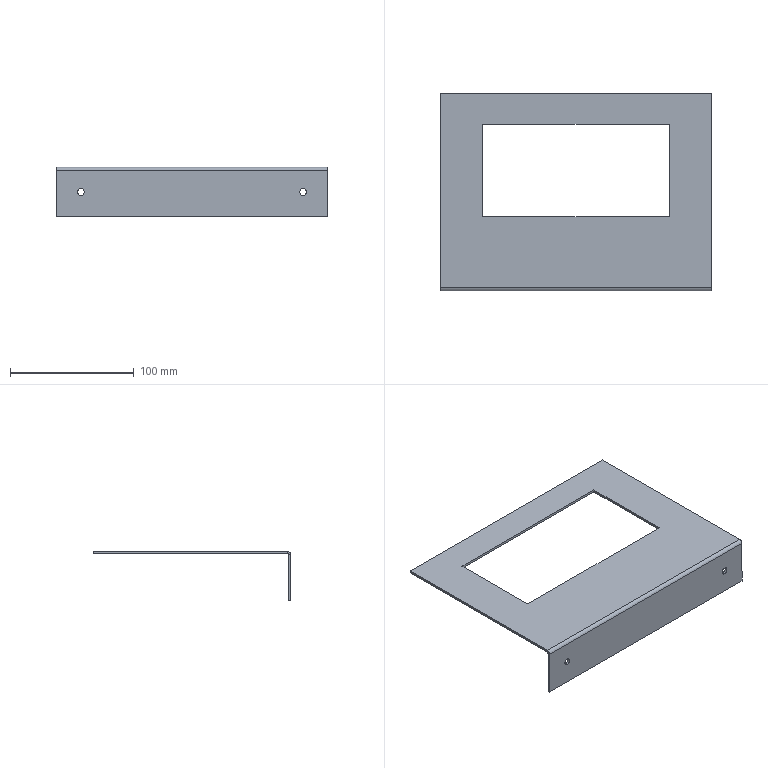Part | STEP file | 1 solid | 22 faces | box 220 x 160 x 40 mm | volume 64047 mm3 | plane 16 | cylinder 6 | commonest cylinder face diameters 5.5 x4 1.473 x1 5.473 x1
STEP:
#1=CARTESIAN_POINT('',(0.,0.,0.));
#2=DIRECTION('',(0.,0.,1.));
#3=DIRECTION('',(1.,0.,0.));
#4=AXIS2_PLACEMENT_3D('',#1,#2,#3);
#5=CARTESIAN_POINT('',(200.,0.,-17.25));
#6=VERTEX_POINT('',#5);
#7=CARTESIAN_POINT('',(200.,2.,-17.25));
#8=VERTEX_POINT('',#7);
#9=CARTESIAN_POINT('',(200.,2.,-17.25));
#10=DIRECTION('',(0.,1.,0.));
#11=VECTOR('',#10,1.);
#12=LINE('',#9,#11);
#13=CARTESIAN_POINT('',(200.,2.,-20.));
#14=DIRECTION('',(0.,1.,0.));
#15=DIRECTION('',(0.,0.,1.));
#16=AXIS2_PLACEMENT_3D('',#13,#14,#15);
#17=CYLINDRICAL_SURFACE('',#16,2.75);
#18=CARTESIAN_POINT('',(6.283,0.));
#19=DIRECTION('',(0.,1.));
#20=VECTOR('',#19,1.);
#21=LINE('',#18,#20);
#22=(GEOMETRIC_REPRESENTATION_CONTEXT(2)PARAMETRIC_REPRESENTATION_CONTEXT()REPRESENTATION_CONTEXT('',''));
#23=DEFINITIONAL_REPRESENTATION('',(#21),#22);
#24=PCURVE('',#17,#23);
#25=CARTESIAN_POINT('',(200.,2.,-20.));
#26=DIRECTION('',(0.,1.,0.));
#27=DIRECTION('',(0.,0.,1.));
#28=AXIS2_PLACEMENT_3D('',#25,#26,#27);
#29=CYLINDRICAL_SURFACE('',#28,2.75);
#30=CARTESIAN_POINT('',(0.,0.));
#31=DIRECTION('',(0.,1.));
#32=VECTOR('',#31,1.);
#33=LINE('',#30,#32);
#34=(GEOMETRIC_REPRESENTATION_CONTEXT(2)PARAMETRIC_REPRESENTATION_CONTEXT()REPRESENTATION_CONTEXT('',''));
#35=DEFINITIONAL_REPRESENTATION('',(#33),#34);
#36=PCURVE('',#29,#35);
#37=SURFACE_CURVE('',#12,(#24,#36),.PCURVE_S1.);
#38=EDGE_CURVE('',#6,#8,#37,.T.);
#39=ORIENTED_EDGE('',*,*,#38,.T.);
#40=CARTESIAN_POINT('',(200.,2.,-22.75));
#41=VERTEX_POINT('',#40);
#42=CARTESIAN_POINT('',(200.,2.,-20.));
#43=DIRECTION('',(0.,1.,0.));
#44=DIRECTION('',(0.,0.,1.));
#45=AXIS2_PLACEMENT_3D('',#42,#43,#44);
#46=CIRCLE('',#45,2.75);
#47=CARTESIAN_POINT('',(0.,0.));
#48=DIRECTION('',(1.,0.));
#49=VECTOR('',#48,1.);
#50=LINE('',#47,#49);
#51=(GEOMETRIC_REPRESENTATION_CONTEXT(2)PARAMETRIC_REPRESENTATION_CONTEXT()REPRESENTATION_CONTEXT('',''));
#52=DEFINITIONAL_REPRESENTATION('',(#50),#51);
#53=PCURVE('',#17,#52);
#54=CARTESIAN_POINT('',(0.,2.,0.));
#55=DIRECTION('',(0.,1.,0.));
#56=DIRECTION('',(0.,0.,1.));
#57=AXIS2_PLACEMENT_3D('',#54,#55,#56);
#58=PLANE('',#57);
#59=CARTESIAN_POINT('',(-20.,200.));
#60=DIRECTION('',(1.,0.));
#61=AXIS2_PLACEMENT_2D('',#59,#60);
#62=CIRCLE('',#61,2.75);
#63=(GEOMETRIC_REPRESENTATION_CONTEXT(2)PARAMETRIC_REPRESENTATION_CONTEXT()REPRESENTATION_CONTEXT('',''));
#64=DEFINITIONAL_REPRESENTATION('',(#62),#63);
#65=PCURVE('',#58,#64);
#66=SURFACE_CURVE('',#46,(#53,#65),.PCURVE_S1.);
#67=EDGE_CURVE('',#41,#8,#66,.T.);
#68=ORIENTED_EDGE('',*,*,#67,.F.);
#69=CARTESIAN_POINT('',(200.,0.,-22.75));
#70=VERTEX_POINT('',#69);
#71=CARTESIAN_POINT('',(200.,2.,-22.75));
#72=DIRECTION('',(0.,1.,0.));
#73=VECTOR('',#72,1.);
#74=LINE('',#71,#73);
#75=CARTESIAN_POINT('',(3.142,0.));
#76=DIRECTION('',(0.,1.));
#77=VECTOR('',#76,1.);
#78=LINE('',#75,#77);
#79=(GEOMETRIC_REPRESENTATION_CONTEXT(2)PARAMETRIC_REPRESENTATION_CONTEXT()REPRESENTATION_CONTEXT('',''));
#80=DEFINITIONAL_REPRESENTATION('',(#78),#79);
#81=PCURVE('',#17,#80);
#82=CARTESIAN_POINT('',(3.142,0.));
#83=DIRECTION('',(0.,1.));
#84=VECTOR('',#83,1.);
#85=LINE('',#82,#84);
#86=(GEOMETRIC_REPRESENTATION_CONTEXT(2)PARAMETRIC_REPRESENTATION_CONTEXT()REPRESENTATION_CONTEXT('',''));
#87=DEFINITIONAL_REPRESENTATION('',(#85),#86);
#88=PCURVE('',#29,#87);
#89=SURFACE_CURVE('',#74,(#81,#88),.PCURVE_S1.);
#90=EDGE_CURVE('',#70,#41,#89,.T.);
#91=ORIENTED_EDGE('',*,*,#90,.F.);
#92=CARTESIAN_POINT('',(200.,0.,-20.));
#93=DIRECTION('',(0.,1.,0.));
#94=DIRECTION('',(0.,0.,1.));
#95=AXIS2_PLACEMENT_3D('',#92,#93,#94);
#96=CIRCLE('',#95,2.75);
#97=CARTESIAN_POINT('',(0.,-2.));
#98=DIRECTION('',(1.,0.));
#99=VECTOR('',#98,1.);
#100=LINE('',#97,#99);
#101=(GEOMETRIC_REPRESENTATION_CONTEXT(2)PARAMETRIC_REPRESENTATION_CONTEXT()REPRESENTATION_CONTEXT('',''));
#102=DEFINITIONAL_REPRESENTATION('',(#100),#101);
#103=PCURVE('',#17,#102);
#104=CARTESIAN_POINT('',(0.,0.,0.));
#105=DIRECTION('',(0.,1.,0.));
#106=DIRECTION('',(0.,0.,1.));
#107=AXIS2_PLACEMENT_3D('',#104,#105,#106);
#108=PLANE('',#107);
#109=CARTESIAN_POINT('',(-20.,200.));
#110=DIRECTION('',(1.,0.));
#111=AXIS2_PLACEMENT_2D('',#109,#110);
#112=CIRCLE('',#111,2.75);
#113=(GEOMETRIC_REPRESENTATION_CONTEXT(2)PARAMETRIC_REPRESENTATION_CONTEXT()REPRESENTATION_CONTEXT('',''));
#114=DEFINITIONAL_REPRESENTATION('',(#112),#113);
#115=PCURVE('',#108,#114);
#116=SURFACE_CURVE('',#96,(#103,#115),.PCURVE_S1.);
#117=EDGE_CURVE('',#70,#6,#116,.T.);
#118=ORIENTED_EDGE('',*,*,#117,.T.);
#119=EDGE_LOOP('',(#39,#68,#91,#118));
#120=FACE_BOUND('',#119,.F.);
#121=ADVANCED_FACE('',(#120),#17,.F.);
#122=CARTESIAN_POINT('',(20.,0.,-17.25));
#123=VERTEX_POINT('',#122);
#124=CARTESIAN_POINT('',(20.,2.,-17.25));
#125=VERTEX_POINT('',#124);
#126=CARTESIAN_POINT('',(20.,2.,-17.25));
#127=DIRECTION('',(0.,1.,0.));
#128=VECTOR('',#127,1.);
#129=LINE('',#126,#128);
#130=CARTESIAN_POINT('',(20.,2.,-20.));
#131=DIRECTION('',(0.,1.,0.));
#132=DIRECTION('',(0.,0.,1.));
#133=AXIS2_PLACEMENT_3D('',#130,#131,#132);
#134=CYLINDRICAL_SURFACE('',#133,2.75);
#135=CARTESIAN_POINT('',(6.283,0.));
#136=DIRECTION('',(0.,1.));
#137=VECTOR('',#136,1.);
#138=LINE('',#135,#137);
#139=(GEOMETRIC_REPRESENTATION_CONTEXT(2)PARAMETRIC_REPRESENTATION_CONTEXT()REPRESENTATION_CONTEXT('',''));
#140=DEFINITIONAL_REPRESENTATION('',(#138),#139);
#141=PCURVE('',#134,#140);
#142=CARTESIAN_POINT('',(20.,2.,-20.));
#143=DIRECTION('',(0.,1.,0.));
#144=DIRECTION('',(0.,0.,1.));
#145=AXIS2_PLACEMENT_3D('',#142,#143,#144);
#146=CYLINDRICAL_SURFACE('',#145,2.75);
#147=CARTESIAN_POINT('',(0.,0.));
#148=DIRECTION('',(0.,1.));
#149=VECTOR('',#148,1.);
#150=LINE('',#147,#149);
#151=(GEOMETRIC_REPRESENTATION_CONTEXT(2)PARAMETRIC_REPRESENTATION_CONTEXT()REPRESENTATION_CONTEXT('',''));
#152=DEFINITIONAL_REPRESENTATION('',(#150),#151);
#153=PCURVE('',#146,#152);
#154=SURFACE_CURVE('',#129,(#141,#153),.PCURVE_S1.);
#155=EDGE_CURVE('',#123,#125,#154,.T.);
#156=ORIENTED_EDGE('',*,*,#155,.T.);
#157=CARTESIAN_POINT('',(20.,2.,-22.75));
#158=VERTEX_POINT('',#157);
#159=CARTESIAN_POINT('',(20.,2.,-20.));
#160=DIRECTION('',(0.,1.,0.));
#161=DIRECTION('',(0.,0.,1.));
#162=AXIS2_PLACEMENT_3D('',#159,#160,#161);
#163=CIRCLE('',#162,2.75);
#164=CARTESIAN_POINT('',(0.,0.));
#165=DIRECTION('',(1.,0.));
#166=VECTOR('',#165,1.);
#167=LINE('',#164,#166);
#168=(GEOMETRIC_REPRESENTATION_CONTEXT(2)PARAMETRIC_REPRESENTATION_CONTEXT()REPRESENTATION_CONTEXT('',''));
#169=DEFINITIONAL_REPRESENTATION('',(#167),#168);
#170=PCURVE('',#134,#169);
#171=CARTESIAN_POINT('',(-20.,20.));
#172=DIRECTION('',(1.,0.));
#173=AXIS2_PLACEMENT_2D('',#171,#172);
#174=CIRCLE('',#173,2.75);
#175=(GEOMETRIC_REPRESENTATION_CONTEXT(2)PARAMETRIC_REPRESENTATION_CONTEXT()REPRESENTATION_CONTEXT('',''));
#176=DEFINITIONAL_REPRESENTATION('',(#174),#175);
#177=PCURVE('',#58,#176);
#178=SURFACE_CURVE('',#163,(#170,#177),.PCURVE_S1.);
#179=EDGE_CURVE('',#158,#125,#178,.T.);
#180=ORIENTED_EDGE('',*,*,#179,.F.);
#181=CARTESIAN_POINT('',(20.,0.,-22.75));
#182=VERTEX_POINT('',#181);
#183=CARTESIAN_POINT('',(20.,2.,-22.75));
#184=DIRECTION('',(0.,1.,0.));
#185=VECTOR('',#184,1.);
#186=LINE('',#183,#185);
#187=CARTESIAN_POINT('',(3.142,0.));
#188=DIRECTION('',(0.,1.));
#189=VECTOR('',#188,1.);
#190=LINE('',#187,#189);
#191=(GEOMETRIC_REPRESENTATION_CONTEXT(2)PARAMETRIC_REPRESENTATION_CONTEXT()REPRESENTATION_CONTEXT('',''));
#192=DEFINITIONAL_REPRESENTATION('',(#190),#191);
#193=PCURVE('',#134,#192);
#194=CARTESIAN_POINT('',(3.142,0.));
#195=DIRECTION('',(0.,1.));
#196=VECTOR('',#195,1.);
#197=LINE('',#194,#196);
#198=(GEOMETRIC_REPRESENTATION_CONTEXT(2)PARAMETRIC_REPRESENTATION_CONTEXT()REPRESENTATION_CONTEXT('',''));
#199=DEFINITIONAL_REPRESENTATION('',(#197),#198);
#200=PCURVE('',#146,#199);
#201=SURFACE_CURVE('',#186,(#193,#200),.PCURVE_S1.);
#202=EDGE_CURVE('',#182,#158,#201,.T.);
#203=ORIENTED_EDGE('',*,*,#202,.F.);
#204=CARTESIAN_POINT('',(20.,0.,-20.));
#205=DIRECTION('',(0.,1.,0.));
#206=DIRECTION('',(0.,0.,1.));
#207=AXIS2_PLACEMENT_3D('',#204,#205,#206);
#208=CIRCLE('',#207,2.75);
#209=CARTESIAN_POINT('',(0.,-2.));
#210=DIRECTION('',(1.,0.));
#211=VECTOR('',#210,1.);
#212=LINE('',#209,#211);
#213=(GEOMETRIC_REPRESENTATION_CONTEXT(2)PARAMETRIC_REPRESENTATION_CONTEXT()REPRESENTATION_CONTEXT('',''));
#214=DEFINITIONAL_REPRESENTATION('',(#212),#213);
#215=PCURVE('',#134,#214);
#216=CARTESIAN_POINT('',(-20.,20.));
#217=DIRECTION('',(1.,0.));
#218=AXIS2_PLACEMENT_2D('',#216,#217);
#219=CIRCLE('',#218,2.75);
#220=(GEOMETRIC_REPRESENTATION_CONTEXT(2)PARAMETRIC_REPRESENTATION_CONTEXT()REPRESENTATION_CONTEXT('',''));
#221=DEFINITIONAL_REPRESENTATION('',(#219),#220);
#222=PCURVE('',#108,#221);
#223=SURFACE_CURVE('',#208,(#215,#222),.PCURVE_S1.);
#224=EDGE_CURVE('',#182,#123,#223,.T.);
#225=ORIENTED_EDGE('',*,*,#224,.T.);
#226=EDGE_LOOP('',(#156,#180,#203,#225));
#227=FACE_BOUND('',#226,.F.);
#228=ADVANCED_FACE('',(#227),#134,.F.);
#229=CARTESIAN_POINT('',(0.,160.,-2.));
#230=VERTEX_POINT('',#229);
#231=CARTESIAN_POINT('',(0.,2.737,-2.));
#232=VERTEX_POINT('',#231);
#233=CARTESIAN_POINT('',(0.,0.,-2.));
#234=DIRECTION('',(0.,-1.,0.));
#235=VECTOR('',#234,1.);
#236=LINE('',#233,#235);
#237=CARTESIAN_POINT('',(0.,0.,-2.));
#238=DIRECTION('',(-1.,0.,0.));
#239=DIRECTION('',(0.,0.,1.));
#240=AXIS2_PLACEMENT_3D('',#237,#238,#239);
#241=PLANE('',#240);
#242=CARTESIAN_POINT('',(0.,0.));
#243=DIRECTION('',(0.,-1.));
#244=VECTOR('',#243,1.);
#245=LINE('',#242,#244);
#246=(GEOMETRIC_REPRESENTATION_CONTEXT(2)PARAMETRIC_REPRESENTATION_CONTEXT()REPRESENTATION_CONTEXT('',''));
#247=DEFINITIONAL_REPRESENTATION('',(#245),#246);
#248=PCURVE('',#241,#247);
#249=CARTESIAN_POINT('',(0.,0.,-2.));
#250=DIRECTION('',(0.,0.,-1.));
#251=DIRECTION('',(-1.,0.,0.));
#252=AXIS2_PLACEMENT_3D('',#249,#250,#251);
#253=PLANE('',#252);
#254=CARTESIAN_POINT('',(0.,0.));
#255=DIRECTION('',(0.,-1.));
#256=VECTOR('',#255,1.);
#257=LINE('',#254,#256);
#258=(GEOMETRIC_REPRESENTATION_CONTEXT(2)PARAMETRIC_REPRESENTATION_CONTEXT()REPRESENTATION_CONTEXT('',''));
#259=DEFINITIONAL_REPRESENTATION('',(#257),#258);
#260=PCURVE('',#253,#259);
#261=SURFACE_CURVE('',#236,(#248,#260),.PCURVE_S1.);
#262=EDGE_CURVE('',#230,#232,#261,.T.);
#263=ORIENTED_EDGE('',*,*,#262,.T.);
#264=CARTESIAN_POINT('',(0.,2.737,0.));
#265=VERTEX_POINT('',#264);
#266=CARTESIAN_POINT('',(0.,2.737,-2.));
#267=DIRECTION('',(0.,0.,1.));
#268=VECTOR('',#267,1.);
#269=LINE('',#266,#268);
#270=CARTESIAN_POINT('',(0.,2.737));
#271=DIRECTION('',(1.,0.));
#272=VECTOR('',#271,1.);
#273=LINE('',#270,#272);
#274=(GEOMETRIC_REPRESENTATION_CONTEXT(2)PARAMETRIC_REPRESENTATION_CONTEXT()REPRESENTATION_CONTEXT('',''));
#275=DEFINITIONAL_REPRESENTATION('',(#273),#274);
#276=PCURVE('',#241,#275);
#277=CARTESIAN_POINT('',(0.,2.737,-2.737));
#278=DIRECTION('',(1.,0.,0.));
#279=DIRECTION('',(0.,0.,-1.));
#280=AXIS2_PLACEMENT_3D('',#277,#278,#279);
#281=PLANE('',#280);
#282=CARTESIAN_POINT('',(-0.7366,0.));
#283=DIRECTION('',(-1.,0.));
#284=VECTOR('',#283,1.);
#285=LINE('',#282,#284);
#286=(GEOMETRIC_REPRESENTATION_CONTEXT(2)PARAMETRIC_REPRESENTATION_CONTEXT()REPRESENTATION_CONTEXT('',''));
#287=DEFINITIONAL_REPRESENTATION('',(#285),#286);
#288=PCURVE('',#281,#287);
#289=SURFACE_CURVE('',#269,(#276,#288),.PCURVE_S1.);
#290=EDGE_CURVE('',#232,#265,#289,.T.);
#291=ORIENTED_EDGE('',*,*,#290,.T.);
#292=CARTESIAN_POINT('',(0.,160.,0.));
#293=VERTEX_POINT('',#292);
#294=CARTESIAN_POINT('',(0.,0.,0.));
#295=DIRECTION('',(0.,-1.,0.));
#296=VECTOR('',#295,1.);
#297=LINE('',#294,#296);
#298=CARTESIAN_POINT('',(2.,0.));
#299=DIRECTION('',(0.,-1.));
#300=VECTOR('',#299,1.);
#301=LINE('',#298,#300);
#302=(GEOMETRIC_REPRESENTATION_CONTEXT(2)PARAMETRIC_REPRESENTATION_CONTEXT()REPRESENTATION_CONTEXT('',''));
#303=DEFINITIONAL_REPRESENTATION('',(#301),#302);
#304=PCURVE('',#241,#303);
#305=CARTESIAN_POINT('',(0.,0.,0.));
#306=DIRECTION('',(0.,0.,-1.));
#307=DIRECTION('',(-1.,0.,0.));
#308=AXIS2_PLACEMENT_3D('',#305,#306,#307);
#309=PLANE('',#308);
#310=CARTESIAN_POINT('',(0.,0.));
#311=DIRECTION('',(0.,-1.));
#312=VECTOR('',#311,1.);
#313=LINE('',#310,#312);
#314=(GEOMETRIC_REPRESENTATION_CONTEXT(2)PARAMETRIC_REPRESENTATION_CONTEXT()REPRESENTATION_CONTEXT('',''));
#315=DEFINITIONAL_REPRESENTATION('',(#313),#314);
#316=PCURVE('',#309,#315);
#317=SURFACE_CURVE('',#297,(#304,#316),.PCURVE_S1.);
#318=EDGE_CURVE('',#293,#265,#317,.T.);
#319=ORIENTED_EDGE('',*,*,#318,.F.);
#320=CARTESIAN_POINT('',(0.,160.,-2.));
#321=DIRECTION('',(0.,0.,1.));
#322=VECTOR('',#321,1.);
#323=LINE('',#320,#322);
#324=CARTESIAN_POINT('',(0.,160.));
#325=DIRECTION('',(1.,0.));
#326=VECTOR('',#325,1.);
#327=LINE('',#324,#326);
#328=(GEOMETRIC_REPRESENTATION_CONTEXT(2)PARAMETRIC_REPRESENTATION_CONTEXT()REPRESENTATION_CONTEXT('',''));
#329=DEFINITIONAL_REPRESENTATION('',(#327),#328);
#330=PCURVE('',#241,#329);
#331=CARTESIAN_POINT('',(0.,160.,-2.));
#332=DIRECTION('',(0.,1.,0.));
#333=DIRECTION('',(0.,0.,1.));
#334=AXIS2_PLACEMENT_3D('',#331,#332,#333);
#335=PLANE('',#334);
#336=CARTESIAN_POINT('',(0.,0.));
#337=DIRECTION('',(1.,0.));
#338=VECTOR('',#337,1.);
#339=LINE('',#336,#338);
#340=(GEOMETRIC_REPRESENTATION_CONTEXT(2)PARAMETRIC_REPRESENTATION_CONTEXT()REPRESENTATION_CONTEXT('',''));
#341=DEFINITIONAL_REPRESENTATION('',(#339),#340);
#342=PCURVE('',#335,#341);
#343=SURFACE_CURVE('',#323,(#330,#342),.PCURVE_S1.);
#344=EDGE_CURVE('',#230,#293,#343,.T.);
#345=ORIENTED_EDGE('',*,*,#344,.F.);
#346=EDGE_LOOP('',(#263,#291,#319,#345));
#347=FACE_BOUND('',#346,.T.);
#348=ADVANCED_FACE('',(#347),#241,.T.);
#349=CARTESIAN_POINT('',(34.5,135.,-2.));
#350=VERTEX_POINT('',#349);
#351=CARTESIAN_POINT('',(34.5,60.,-2.));
#352=VERTEX_POINT('',#351);
#353=CARTESIAN_POINT('',(34.5,135.,-2.));
#354=DIRECTION('',(0.,-1.,0.));
#355=VECTOR('',#354,1.);
#356=LINE('',#353,#355);
#357=CARTESIAN_POINT('',(-34.5,135.));
#358=DIRECTION('',(0.,-1.));
#359=VECTOR('',#358,1.);
#360=LINE('',#357,#359);
#361=(GEOMETRIC_REPRESENTATION_CONTEXT(2)PARAMETRIC_REPRESENTATION_CONTEXT()REPRESENTATION_CONTEXT('',''));
#362=DEFINITIONAL_REPRESENTATION('',(#360),#361);
#363=PCURVE('',#253,#362);
#364=CARTESIAN_POINT('',(34.5,135.,-2.));
#365=DIRECTION('',(-1.,0.,0.));
#366=DIRECTION('',(0.,-1.,0.));
#367=AXIS2_PLACEMENT_3D('',#364,#365,#366);
#368=PLANE('',#367);
#369=CARTESIAN_POINT('',(0.,0.));
#370=DIRECTION('',(1.,0.));
#371=VECTOR('',#370,1.);
#372=LINE('',#369,#371);
#373=(GEOMETRIC_REPRESENTATION_CONTEXT(2)PARAMETRIC_REPRESENTATION_CONTEXT()REPRESENTATION_CONTEXT('',''));
#374=DEFINITIONAL_REPRESENTATION('',(#372),#373);
#375=PCURVE('',#368,#374);
#376=SURFACE_CURVE('',#356,(#363,#375),.PCURVE_S1.);
#377=EDGE_CURVE('',#350,#352,#376,.T.);
#378=ORIENTED_EDGE('',*,*,#377,.T.);
#379=CARTESIAN_POINT('',(185.5,60.,-2.));
#380=VERTEX_POINT('',#379);
#381=CARTESIAN_POINT('',(34.5,60.,-2.));
#382=DIRECTION('',(1.,0.,0.));
#383=VECTOR('',#382,1.);
#384=LINE('',#381,#383);
#385=CARTESIAN_POINT('',(-34.5,60.));
#386=DIRECTION('',(-1.,0.));
#387=VECTOR('',#386,1.);
#388=LINE('',#385,#387);
#389=(GEOMETRIC_REPRESENTATION_CONTEXT(2)PARAMETRIC_REPRESENTATION_CONTEXT()REPRESENTATION_CONTEXT('',''));
#390=DEFINITIONAL_REPRESENTATION('',(#388),#389);
#391=PCURVE('',#253,#390);
#392=CARTESIAN_POINT('',(34.5,60.,-2.));
#393=DIRECTION('',(0.,-1.,0.));
#394=DIRECTION('',(0.,0.,-1.));
#395=AXIS2_PLACEMENT_3D('',#392,#393,#394);
#396=PLANE('',#395);
#397=CARTESIAN_POINT('',(0.,0.));
#398=DIRECTION('',(0.,1.));
#399=VECTOR('',#398,1.);
#400=LINE('',#397,#399);
#401=(GEOMETRIC_REPRESENTATION_CONTEXT(2)PARAMETRIC_REPRESENTATION_CONTEXT()REPRESENTATION_CONTEXT('',''));
#402=DEFINITIONAL_REPRESENTATION('',(#400),#401);
#403=PCURVE('',#396,#402);
#404=SURFACE_CURVE('',#384,(#391,#403),.PCURVE_S1.);
#405=EDGE_CURVE('',#352,#380,#404,.T.);
#406=ORIENTED_EDGE('',*,*,#405,.T.);
#407=CARTESIAN_POINT('',(185.5,135.,-2.));
#408=VERTEX_POINT('',#407);
#409=CARTESIAN_POINT('',(185.5,135.,-2.));
#410=DIRECTION('',(0.,1.,0.));
#411=VECTOR('',#410,1.);
#412=LINE('',#409,#411);
#413=CARTESIAN_POINT('',(-185.5,135.));
#414=DIRECTION('',(0.,1.));
#415=VECTOR('',#414,1.);
#416=LINE('',#413,#415);
#417=(GEOMETRIC_REPRESENTATION_CONTEXT(2)PARAMETRIC_REPRESENTATION_CONTEXT()REPRESENTATION_CONTEXT('',''));
#418=DEFINITIONAL_REPRESENTATION('',(#416),#417);
#419=PCURVE('',#253,#418);
#420=CARTESIAN_POINT('',(185.5,135.,-2.));
#421=DIRECTION('',(1.,0.,0.));
#422=DIRECTION('',(0.,0.,-1.));
#423=AXIS2_PLACEMENT_3D('',#420,#421,#422);
#424=PLANE('',#423);
#425=CARTESIAN_POINT('',(0.,0.));
#426=DIRECTION('',(0.,1.));
#427=VECTOR('',#426,1.);
#428=LINE('',#425,#427);
#429=(GEOMETRIC_REPRESENTATION_CONTEXT(2)PARAMETRIC_REPRESENTATION_CONTEXT()REPRESENTATION_CONTEXT('',''));
#430=DEFINITIONAL_REPRESENTATION('',(#428),#429);
#431=PCURVE('',#424,#430);
#432=SURFACE_CURVE('',#412,(#419,#431),.PCURVE_S1.);
#433=EDGE_CURVE('',#380,#408,#432,.T.);
#434=ORIENTED_EDGE('',*,*,#433,.T.);
#435=CARTESIAN_POINT('',(34.5,135.,-2.));
#436=DIRECTION('',(-1.,0.,0.));
#437=VECTOR('',#436,1.);
#438=LINE('',#435,#437);
#439=CARTESIAN_POINT('',(-34.5,135.));
#440=DIRECTION('',(1.,0.));
#441=VECTOR('',#440,1.);
#442=LINE('',#439,#441);
#443=(GEOMETRIC_REPRESENTATION_CONTEXT(2)PARAMETRIC_REPRESENTATION_CONTEXT()REPRESENTATION_CONTEXT('',''));
#444=DEFINITIONAL_REPRESENTATION('',(#442),#443);
#445=PCURVE('',#253,#444);
#446=CARTESIAN_POINT('',(34.5,135.,-2.));
#447=DIRECTION('',(0.,1.,0.));
#448=DIRECTION('',(0.,0.,1.));
#449=AXIS2_PLACEMENT_3D('',#446,#447,#448);
#450=PLANE('',#449);
#451=CARTESIAN_POINT('',(0.,0.));
#452=DIRECTION('',(0.,-1.));
#453=VECTOR('',#452,1.);
#454=LINE('',#451,#453);
#455=(GEOMETRIC_REPRESENTATION_CONTEXT(2)PARAMETRIC_REPRESENTATION_CONTEXT()REPRESENTATION_CONTEXT('',''));
#456=DEFINITIONAL_REPRESENTATION('',(#454),#455);
#457=PCURVE('',#450,#456);
#458=SURFACE_CURVE('',#438,(#445,#457),.PCURVE_S1.);
#459=EDGE_CURVE('',#408,#350,#458,.T.);
#460=ORIENTED_EDGE('',*,*,#459,.T.);
#461=EDGE_LOOP('',(#378,#406,#434,#460));
#462=FACE_BOUND('',#461,.T.);
#463=CARTESIAN_POINT('',(220.,2.737,-2.));
#464=VERTEX_POINT('',#463);
#465=CARTESIAN_POINT('',(220.,160.,-2.));
#466=VERTEX_POINT('',#465);
#467=CARTESIAN_POINT('',(220.,0.,-2.));
#468=DIRECTION('',(0.,1.,0.));
#469=VECTOR('',#468,1.);
#470=LINE('',#467,#469);
#471=CARTESIAN_POINT('',(-220.,0.));
#472=DIRECTION('',(0.,1.));
#473=VECTOR('',#472,1.);
#474=LINE('',#471,#473);
#475=(GEOMETRIC_REPRESENTATION_CONTEXT(2)PARAMETRIC_REPRESENTATION_CONTEXT()REPRESENTATION_CONTEXT('',''));
#476=DEFINITIONAL_REPRESENTATION('',(#474),#475);
#477=PCURVE('',#253,#476);
#478=CARTESIAN_POINT('',(220.,0.,-2.));
#479=DIRECTION('',(1.,0.,0.));
#480=DIRECTION('',(0.,0.,-1.));
#481=AXIS2_PLACEMENT_3D('',#478,#479,#480);
#482=PLANE('',#481);
#483=CARTESIAN_POINT('',(0.,0.));
#484=DIRECTION('',(0.,1.));
#485=VECTOR('',#484,1.);
#486=LINE('',#483,#485);
#487=(GEOMETRIC_REPRESENTATION_CONTEXT(2)PARAMETRIC_REPRESENTATION_CONTEXT()REPRESENTATION_CONTEXT('',''));
#488=DEFINITIONAL_REPRESENTATION('',(#486),#487);
#489=PCURVE('',#482,#488);
#490=SURFACE_CURVE('',#470,(#477,#489),.PCURVE_S1.);
#491=EDGE_CURVE('',#464,#466,#490,.T.);
#492=ORIENTED_EDGE('',*,*,#491,.F.);
#493=CARTESIAN_POINT('',(0.,2.737,-2.));
#494=DIRECTION('',(1.,0.,0.));
#495=VECTOR('',#494,1.);
#496=LINE('',#493,#495);
#497=CARTESIAN_POINT('',(0.,2.737));
#498=DIRECTION('',(-1.,0.));
#499=VECTOR('',#498,1.);
#500=LINE('',#497,#499);
#501=(GEOMETRIC_REPRESENTATION_CONTEXT(2)PARAMETRIC_REPRESENTATION_CONTEXT()REPRESENTATION_CONTEXT('',''));
#502=DEFINITIONAL_REPRESENTATION('',(#500),#501);
#503=PCURVE('',#253,#502);
#504=CARTESIAN_POINT('',(0.,2.737,-2.737));
#505=DIRECTION('',(-1.,0.,0.));
#506=DIRECTION('',(0.,-1.,0.));
#507=AXIS2_PLACEMENT_3D('',#504,#505,#506);
#508=CYLINDRICAL_SURFACE('',#507,0.7366);
#509=CARTESIAN_POINT('',(1.571,0.));
#510=DIRECTION('',(0.,-1.));
#511=VECTOR('',#510,1.);
#512=LINE('',#509,#511);
#513=(GEOMETRIC_REPRESENTATION_CONTEXT(2)PARAMETRIC_REPRESENTATION_CONTEXT()REPRESENTATION_CONTEXT('',''));
#514=DEFINITIONAL_REPRESENTATION('',(#512),#513);
#515=PCURVE('',#508,#514);
#516=SURFACE_CURVE('',#496,(#503,#515),.PCURVE_S1.);
#517=EDGE_CURVE('',#232,#464,#516,.T.);
#518=ORIENTED_EDGE('',*,*,#517,.F.);
#519=ORIENTED_EDGE('',*,*,#262,.F.);
#520=CARTESIAN_POINT('',(0.,160.,-2.));
#521=DIRECTION('',(-1.,0.,0.));
#522=VECTOR('',#521,1.);
#523=LINE('',#520,#522);
#524=CARTESIAN_POINT('',(0.,160.));
#525=DIRECTION('',(1.,0.));
#526=VECTOR('',#525,1.);
#527=LINE('',#524,#526);
#528=(GEOMETRIC_REPRESENTATION_CONTEXT(2)PARAMETRIC_REPRESENTATION_CONTEXT()REPRESENTATION_CONTEXT('',''));
#529=DEFINITIONAL_REPRESENTATION('',(#527),#528);
#530=PCURVE('',#253,#529);
#531=CARTESIAN_POINT('',(0.,0.));
#532=DIRECTION('',(0.,-1.));
#533=VECTOR('',#532,1.);
#534=LINE('',#531,#533);
#535=(GEOMETRIC_REPRESENTATION_CONTEXT(2)PARAMETRIC_REPRESENTATION_CONTEXT()REPRESENTATION_CONTEXT('',''));
#536=DEFINITIONAL_REPRESENTATION('',(#534),#535);
#537=PCURVE('',#335,#536);
#538=SURFACE_CURVE('',#523,(#530,#537),.PCURVE_S1.);
#539=EDGE_CURVE('',#466,#230,#538,.T.);
#540=ORIENTED_EDGE('',*,*,#539,.F.);
#541=EDGE_LOOP('',(#492,#518,#519,#540));
#542=FACE_BOUND('',#541,.T.);
#543=ADVANCED_FACE('',(#462,#542),#253,.T.);
#544=CARTESIAN_POINT('',(34.5,60.,0.));
#545=VERTEX_POINT('',#544);
#546=CARTESIAN_POINT('',(185.5,60.,0.));
#547=VERTEX_POINT('',#546);
#548=CARTESIAN_POINT('',(34.5,60.,0.));
#549=DIRECTION('',(1.,0.,0.));
#550=VECTOR('',#549,1.);
#551=LINE('',#548,#550);
#552=CARTESIAN_POINT('',(-34.5,60.));
#553=DIRECTION('',(-1.,0.));
#554=VECTOR('',#553,1.);
#555=LINE('',#552,#554);
#556=(GEOMETRIC_REPRESENTATION_CONTEXT(2)PARAMETRIC_REPRESENTATION_CONTEXT()REPRESENTATION_CONTEXT('',''));
#557=DEFINITIONAL_REPRESENTATION('',(#555),#556);
#558=PCURVE('',#309,#557);
#559=CARTESIAN_POINT('',(-2.,0.));
#560=DIRECTION('',(0.,1.));
#561=VECTOR('',#560,1.);
#562=LINE('',#559,#561);
#563=(GEOMETRIC_REPRESENTATION_CONTEXT(2)PARAMETRIC_REPRESENTATION_CONTEXT()REPRESENTATION_CONTEXT('',''));
#564=DEFINITIONAL_REPRESENTATION('',(#562),#563);
#565=PCURVE('',#396,#564);
#566=SURFACE_CURVE('',#551,(#558,#565),.PCURVE_S1.);
#567=EDGE_CURVE('',#545,#547,#566,.T.);
#568=ORIENTED_EDGE('',*,*,#567,.F.);
#569=CARTESIAN_POINT('',(34.5,135.,0.));
#570=VERTEX_POINT('',#569);
#571=CARTESIAN_POINT('',(34.5,135.,0.));
#572=DIRECTION('',(0.,-1.,0.));
#573=VECTOR('',#572,1.);
#574=LINE('',#571,#573);
#575=CARTESIAN_POINT('',(-34.5,135.));
#576=DIRECTION('',(0.,-1.));
#577=VECTOR('',#576,1.);
#578=LINE('',#575,#577);
#579=(GEOMETRIC_REPRESENTATION_CONTEXT(2)PARAMETRIC_REPRESENTATION_CONTEXT()REPRESENTATION_CONTEXT('',''));
#580=DEFINITIONAL_REPRESENTATION('',(#578),#579);
#581=PCURVE('',#309,#580);
#582=CARTESIAN_POINT('',(0.,2.));
#583=DIRECTION('',(1.,0.));
#584=VECTOR('',#583,1.);
#585=LINE('',#582,#584);
#586=(GEOMETRIC_REPRESENTATION_CONTEXT(2)PARAMETRIC_REPRESENTATION_CONTEXT()REPRESENTATION_CONTEXT('',''));
#587=DEFINITIONAL_REPRESENTATION('',(#585),#586);
#588=PCURVE('',#368,#587);
#589=SURFACE_CURVE('',#574,(#581,#588),.PCURVE_S1.);
#590=EDGE_CURVE('',#570,#545,#589,.T.);
#591=ORIENTED_EDGE('',*,*,#590,.F.);
#592=CARTESIAN_POINT('',(185.5,135.,0.));
#593=VERTEX_POINT('',#592);
#594=CARTESIAN_POINT('',(34.5,135.,0.));
#595=DIRECTION('',(-1.,0.,0.));
#596=VECTOR('',#595,1.);
#597=LINE('',#594,#596);
#598=CARTESIAN_POINT('',(-34.5,135.));
#599=DIRECTION('',(1.,0.));
#600=VECTOR('',#599,1.);
#601=LINE('',#598,#600);
#602=(GEOMETRIC_REPRESENTATION_CONTEXT(2)PARAMETRIC_REPRESENTATION_CONTEXT()REPRESENTATION_CONTEXT('',''));
#603=DEFINITIONAL_REPRESENTATION('',(#601),#602);
#604=PCURVE('',#309,#603);
#605=CARTESIAN_POINT('',(2.,0.));
#606=DIRECTION('',(0.,-1.));
#607=VECTOR('',#606,1.);
#608=LINE('',#605,#607);
#609=(GEOMETRIC_REPRESENTATION_CONTEXT(2)PARAMETRIC_REPRESENTATION_CONTEXT()REPRESENTATION_CONTEXT('',''));
#610=DEFINITIONAL_REPRESENTATION('',(#608),#609);
#611=PCURVE('',#450,#610);
#612=SURFACE_CURVE('',#597,(#604,#611),.PCURVE_S1.);
#613=EDGE_CURVE('',#593,#570,#612,.T.);
#614=ORIENTED_EDGE('',*,*,#613,.F.);
#615=CARTESIAN_POINT('',(185.5,135.,0.));
#616=DIRECTION('',(0.,1.,0.));
#617=VECTOR('',#616,1.);
#618=LINE('',#615,#617);
#619=CARTESIAN_POINT('',(-185.5,135.));
#620=DIRECTION('',(0.,1.));
#621=VECTOR('',#620,1.);
#622=LINE('',#619,#621);
#623=(GEOMETRIC_REPRESENTATION_CONTEXT(2)PARAMETRIC_REPRESENTATION_CONTEXT()REPRESENTATION_CONTEXT('',''));
#624=DEFINITIONAL_REPRESENTATION('',(#622),#623);
#625=PCURVE('',#309,#624);
#626=CARTESIAN_POINT('',(-2.,0.));
#627=DIRECTION('',(0.,1.));
#628=VECTOR('',#627,1.);
#629=LINE('',#626,#628);
#630=(GEOMETRIC_REPRESENTATION_CONTEXT(2)PARAMETRIC_REPRESENTATION_CONTEXT()REPRESENTATION_CONTEXT('',''));
#631=DEFINITIONAL_REPRESENTATION('',(#629),#630);
#632=PCURVE('',#424,#631);
#633=SURFACE_CURVE('',#618,(#625,#632),.PCURVE_S1.);
#634=EDGE_CURVE('',#547,#593,#633,.T.);
#635=ORIENTED_EDGE('',*,*,#634,.F.);
#636=EDGE_LOOP('',(#568,#591,#614,#635));
#637=FACE_BOUND('',#636,.T.);
#638=CARTESIAN_POINT('',(220.,2.737,0.));
#639=VERTEX_POINT('',#638);
#640=CARTESIAN_POINT('',(0.,2.737,0.));
#641=DIRECTION('',(1.,0.,0.));
#642=VECTOR('',#641,1.);
#643=LINE('',#640,#642);
#644=CARTESIAN_POINT('',(0.,2.737));
#645=DIRECTION('',(-1.,0.));
#646=VECTOR('',#645,1.);
#647=LINE('',#644,#646);
#648=(GEOMETRIC_REPRESENTATION_CONTEXT(2)PARAMETRIC_REPRESENTATION_CONTEXT()REPRESENTATION_CONTEXT('',''));
#649=DEFINITIONAL_REPRESENTATION('',(#647),#648);
#650=PCURVE('',#309,#649);
#651=CARTESIAN_POINT('',(0.,2.737,-2.737));
#652=DIRECTION('',(-1.,0.,0.));
#653=DIRECTION('',(0.,-1.,0.));
#654=AXIS2_PLACEMENT_3D('',#651,#652,#653);
#655=CYLINDRICAL_SURFACE('',#654,2.737);
#656=CARTESIAN_POINT('',(1.571,0.));
#657=DIRECTION('',(0.,-1.));
#658=VECTOR('',#657,1.);
#659=LINE('',#656,#658);
#660=(GEOMETRIC_REPRESENTATION_CONTEXT(2)PARAMETRIC_REPRESENTATION_CONTEXT()REPRESENTATION_CONTEXT('',''));
#661=DEFINITIONAL_REPRESENTATION('',(#659),#660);
#662=PCURVE('',#655,#661);
#663=SURFACE_CURVE('',#643,(#650,#662),.PCURVE_S1.);
#664=EDGE_CURVE('',#265,#639,#663,.T.);
#665=ORIENTED_EDGE('',*,*,#664,.T.);
#666=CARTESIAN_POINT('',(220.,160.,0.));
#667=VERTEX_POINT('',#666);
#668=CARTESIAN_POINT('',(220.,0.,0.));
#669=DIRECTION('',(0.,1.,0.));
#670=VECTOR('',#669,1.);
#671=LINE('',#668,#670);
#672=CARTESIAN_POINT('',(-220.,0.));
#673=DIRECTION('',(0.,1.));
#674=VECTOR('',#673,1.);
#675=LINE('',#672,#674);
#676=(GEOMETRIC_REPRESENTATION_CONTEXT(2)PARAMETRIC_REPRESENTATION_CONTEXT()REPRESENTATION_CONTEXT('',''));
#677=DEFINITIONAL_REPRESENTATION('',(#675),#676);
#678=PCURVE('',#309,#677);
#679=CARTESIAN_POINT('',(-2.,0.));
#680=DIRECTION('',(0.,1.));
#681=VECTOR('',#680,1.);
#682=LINE('',#679,#681);
#683=(GEOMETRIC_REPRESENTATION_CONTEXT(2)PARAMETRIC_REPRESENTATION_CONTEXT()REPRESENTATION_CONTEXT('',''));
#684=DEFINITIONAL_REPRESENTATION('',(#682),#683);
#685=PCURVE('',#482,#684);
#686=SURFACE_CURVE('',#671,(#678,#685),.PCURVE_S1.);
#687=EDGE_CURVE('',#639,#667,#686,.T.);
#688=ORIENTED_EDGE('',*,*,#687,.T.);
#689=CARTESIAN_POINT('',(0.,160.,0.));
#690=DIRECTION('',(-1.,0.,0.));
#691=VECTOR('',#690,1.);
#692=LINE('',#689,#691);
#693=CARTESIAN_POINT('',(0.,160.));
#694=DIRECTION('',(1.,0.));
#695=VECTOR('',#694,1.);
#696=LINE('',#693,#695);
#697=(GEOMETRIC_REPRESENTATION_CONTEXT(2)PARAMETRIC_REPRESENTATION_CONTEXT()REPRESENTATION_CONTEXT('',''));
#698=DEFINITIONAL_REPRESENTATION('',(#696),#697);
#699=PCURVE('',#309,#698);
#700=CARTESIAN_POINT('',(2.,0.));
#701=DIRECTION('',(0.,-1.));
#702=VECTOR('',#701,1.);
#703=LINE('',#700,#702);
#704=(GEOMETRIC_REPRESENTATION_CONTEXT(2)PARAMETRIC_REPRESENTATION_CONTEXT()REPRESENTATION_CONTEXT('',''));
#705=DEFINITIONAL_REPRESENTATION('',(#703),#704);
#706=PCURVE('',#335,#705);
#707=SURFACE_CURVE('',#692,(#699,#706),.PCURVE_S1.);
#708=EDGE_CURVE('',#667,#293,#707,.T.);
#709=ORIENTED_EDGE('',*,*,#708,.T.);
#710=ORIENTED_EDGE('',*,*,#318,.T.);
#711=EDGE_LOOP('',(#665,#688,#709,#710));
#712=FACE_BOUND('',#711,.T.);
#713=ADVANCED_FACE('',(#637,#712),#309,.F.);
#714=ORIENTED_EDGE('',*,*,#708,.F.);
#715=CARTESIAN_POINT('',(220.,160.,-2.));
#716=DIRECTION('',(0.,0.,1.));
#717=VECTOR('',#716,1.);
#718=LINE('',#715,#717);
#719=CARTESIAN_POINT('',(0.,220.));
#720=DIRECTION('',(1.,0.));
#721=VECTOR('',#720,1.);
#722=LINE('',#719,#721);
#723=(GEOMETRIC_REPRESENTATION_CONTEXT(2)PARAMETRIC_REPRESENTATION_CONTEXT()REPRESENTATION_CONTEXT('',''));
#724=DEFINITIONAL_REPRESENTATION('',(#722),#723);
#725=PCURVE('',#335,#724);
#726=CARTESIAN_POINT('',(0.,160.));
#727=DIRECTION('',(-1.,0.));
#728=VECTOR('',#727,1.);
#729=LINE('',#726,#728);
#730=(GEOMETRIC_REPRESENTATION_CONTEXT(2)PARAMETRIC_REPRESENTATION_CONTEXT()REPRESENTATION_CONTEXT('',''));
#731=DEFINITIONAL_REPRESENTATION('',(#729),#730);
#732=PCURVE('',#482,#731);
#733=SURFACE_CURVE('',#718,(#725,#732),.PCURVE_S1.);
#734=EDGE_CURVE('',#466,#667,#733,.T.);
#735=ORIENTED_EDGE('',*,*,#734,.F.);
#736=ORIENTED_EDGE('',*,*,#539,.T.);
#737=ORIENTED_EDGE('',*,*,#344,.T.);
#738=EDGE_LOOP('',(#714,#735,#736,#737));
#739=FACE_BOUND('',#738,.T.);
#740=ADVANCED_FACE('',(#739),#335,.T.);
#741=CARTESIAN_POINT('',(220.,2.737,-2.));
#742=DIRECTION('',(0.,0.,1.));
#743=VECTOR('',#742,1.);
#744=LINE('',#741,#743);
#745=CARTESIAN_POINT('',(0.,2.737));
#746=DIRECTION('',(-1.,0.));
#747=VECTOR('',#746,1.);
#748=LINE('',#745,#747);
#749=(GEOMETRIC_REPRESENTATION_CONTEXT(2)PARAMETRIC_REPRESENTATION_CONTEXT()REPRESENTATION_CONTEXT('',''));
#750=DEFINITIONAL_REPRESENTATION('',(#748),#749);
#751=PCURVE('',#482,#750);
#752=CARTESIAN_POINT('',(220.,2.737,-2.737));
#753=DIRECTION('',(1.,0.,0.));
#754=DIRECTION('',(0.,0.,-1.));
#755=AXIS2_PLACEMENT_3D('',#752,#753,#754);
#756=PLANE('',#755);
#757=CARTESIAN_POINT('',(-0.7366,0.));
#758=DIRECTION('',(-1.,0.));
#759=VECTOR('',#758,1.);
#760=LINE('',#757,#759);
#761=(GEOMETRIC_REPRESENTATION_CONTEXT(2)PARAMETRIC_REPRESENTATION_CONTEXT()REPRESENTATION_CONTEXT('',''));
#762=DEFINITIONAL_REPRESENTATION('',(#760),#761);
#763=PCURVE('',#756,#762);
#764=SURFACE_CURVE('',#744,(#751,#763),.PCURVE_S1.);
#765=EDGE_CURVE('',#464,#639,#764,.T.);
#766=ORIENTED_EDGE('',*,*,#765,.F.);
#767=ORIENTED_EDGE('',*,*,#491,.T.);
#768=ORIENTED_EDGE('',*,*,#734,.T.);
#769=ORIENTED_EDGE('',*,*,#687,.F.);
#770=EDGE_LOOP('',(#766,#767,#768,#769));
#771=FACE_BOUND('',#770,.T.);
#772=ADVANCED_FACE('',(#771),#482,.T.);
#773=ORIENTED_EDGE('',*,*,#590,.T.);
#774=CARTESIAN_POINT('',(34.5,60.,-2.));
#775=DIRECTION('',(0.,0.,1.));
#776=VECTOR('',#775,1.);
#777=LINE('',#774,#776);
#778=CARTESIAN_POINT('',(75.,0.));
#779=DIRECTION('',(0.,1.));
#780=VECTOR('',#779,1.);
#781=LINE('',#778,#780);
#782=(GEOMETRIC_REPRESENTATION_CONTEXT(2)PARAMETRIC_REPRESENTATION_CONTEXT()REPRESENTATION_CONTEXT('',''));
#783=DEFINITIONAL_REPRESENTATION('',(#781),#782);
#784=PCURVE('',#368,#783);
#785=CARTESIAN_POINT('',(0.,0.));
#786=DIRECTION('',(-1.,0.));
#787=VECTOR('',#786,1.);
#788=LINE('',#785,#787);
#789=(GEOMETRIC_REPRESENTATION_CONTEXT(2)PARAMETRIC_REPRESENTATION_CONTEXT()REPRESENTATION_CONTEXT('',''));
#790=DEFINITIONAL_REPRESENTATION('',(#788),#789);
#791=PCURVE('',#396,#790);
#792=SURFACE_CURVE('',#777,(#784,#791),.PCURVE_S1.);
#793=EDGE_CURVE('',#352,#545,#792,.T.);
#794=ORIENTED_EDGE('',*,*,#793,.F.);
#795=ORIENTED_EDGE('',*,*,#377,.F.);
#796=CARTESIAN_POINT('',(34.5,135.,-2.));
#797=DIRECTION('',(0.,0.,1.));
#798=VECTOR('',#797,1.);
#799=LINE('',#796,#798);
#800=CARTESIAN_POINT('',(0.,0.));
#801=DIRECTION('',(0.,1.));
#802=VECTOR('',#801,1.);
#803=LINE('',#800,#802);
#804=(GEOMETRIC_REPRESENTATION_CONTEXT(2)PARAMETRIC_REPRESENTATION_CONTEXT()REPRESENTATION_CONTEXT('',''));
#805=DEFINITIONAL_REPRESENTATION('',(#803),#804);
#806=PCURVE('',#368,#805);
#807=CARTESIAN_POINT('',(0.,0.));
#808=DIRECTION('',(1.,0.));
#809=VECTOR('',#808,1.);
#810=LINE('',#807,#809);
#811=(GEOMETRIC_REPRESENTATION_CONTEXT(2)PARAMETRIC_REPRESENTATION_CONTEXT()REPRESENTATION_CONTEXT('',''));
#812=DEFINITIONAL_REPRESENTATION('',(#810),#811);
#813=PCURVE('',#450,#812);
#814=SURFACE_CURVE('',#799,(#806,#813),.PCURVE_S1.);
#815=EDGE_CURVE('',#350,#570,#814,.T.);
#816=ORIENTED_EDGE('',*,*,#815,.T.);
#817=EDGE_LOOP('',(#773,#794,#795,#816));
#818=FACE_BOUND('',#817,.T.);
#819=ADVANCED_FACE('',(#818),#368,.F.);
#820=ORIENTED_EDGE('',*,*,#613,.T.);
#821=ORIENTED_EDGE('',*,*,#815,.F.);
#822=ORIENTED_EDGE('',*,*,#459,.F.);
#823=CARTESIAN_POINT('',(185.5,135.,-2.));
#824=DIRECTION('',(0.,0.,1.));
#825=VECTOR('',#824,1.);
#826=LINE('',#823,#825);
#827=CARTESIAN_POINT('',(0.,151.));
#828=DIRECTION('',(1.,0.));
#829=VECTOR('',#828,1.);
#830=LINE('',#827,#829);
#831=(GEOMETRIC_REPRESENTATION_CONTEXT(2)PARAMETRIC_REPRESENTATION_CONTEXT()REPRESENTATION_CONTEXT('',''));
#832=DEFINITIONAL_REPRESENTATION('',(#830),#831);
#833=PCURVE('',#450,#832);
#834=CARTESIAN_POINT('',(0.,0.));
#835=DIRECTION('',(-1.,0.));
#836=VECTOR('',#835,1.);
#837=LINE('',#834,#836);
#838=(GEOMETRIC_REPRESENTATION_CONTEXT(2)PARAMETRIC_REPRESENTATION_CONTEXT()REPRESENTATION_CONTEXT('',''));
#839=DEFINITIONAL_REPRESENTATION('',(#837),#838);
#840=PCURVE('',#424,#839);
#841=SURFACE_CURVE('',#826,(#833,#840),.PCURVE_S1.);
#842=EDGE_CURVE('',#408,#593,#841,.T.);
#843=ORIENTED_EDGE('',*,*,#842,.T.);
#844=EDGE_LOOP('',(#820,#821,#822,#843));
#845=FACE_BOUND('',#844,.T.);
#846=ADVANCED_FACE('',(#845),#450,.F.);
#847=ORIENTED_EDGE('',*,*,#634,.T.);
#848=ORIENTED_EDGE('',*,*,#842,.F.);
#849=ORIENTED_EDGE('',*,*,#433,.F.);
#850=CARTESIAN_POINT('',(185.5,60.,-2.));
#851=DIRECTION('',(0.,0.,1.));
#852=VECTOR('',#851,1.);
#853=LINE('',#850,#852);
#854=CARTESIAN_POINT('',(0.,-75.));
#855=DIRECTION('',(-1.,0.));
#856=VECTOR('',#855,1.);
#857=LINE('',#854,#856);
#858=(GEOMETRIC_REPRESENTATION_CONTEXT(2)PARAMETRIC_REPRESENTATION_CONTEXT()REPRESENTATION_CONTEXT('',''));
#859=DEFINITIONAL_REPRESENTATION('',(#857),#858);
#860=PCURVE('',#424,#859);
#861=CARTESIAN_POINT('',(0.,151.));
#862=DIRECTION('',(-1.,0.));
#863=VECTOR('',#862,1.);
#864=LINE('',#861,#863);
#865=(GEOMETRIC_REPRESENTATION_CONTEXT(2)PARAMETRIC_REPRESENTATION_CONTEXT()REPRESENTATION_CONTEXT('',''));
#866=DEFINITIONAL_REPRESENTATION('',(#864),#865);
#867=PCURVE('',#396,#866);
#868=SURFACE_CURVE('',#853,(#860,#867),.PCURVE_S1.);
#869=EDGE_CURVE('',#380,#547,#868,.T.);
#870=ORIENTED_EDGE('',*,*,#869,.T.);
#871=EDGE_LOOP('',(#847,#848,#849,#870));
#872=FACE_BOUND('',#871,.T.);
#873=ADVANCED_FACE('',(#872),#424,.F.);
#874=ORIENTED_EDGE('',*,*,#567,.T.);
#875=ORIENTED_EDGE('',*,*,#869,.F.);
#876=ORIENTED_EDGE('',*,*,#405,.F.);
#877=ORIENTED_EDGE('',*,*,#793,.T.);
#878=EDGE_LOOP('',(#874,#875,#876,#877));
#879=FACE_BOUND('',#878,.T.);
#880=ADVANCED_FACE('',(#879),#396,.F.);
#881=CARTESIAN_POINT('',(220.,2.,-2.737));
#882=VERTEX_POINT('',#881);
#883=CARTESIAN_POINT('',(220.,0.,-2.737));
#884=VERTEX_POINT('',#883);
#885=CARTESIAN_POINT('',(220.,0.,-2.737));
#886=DIRECTION('',(0.,-1.,0.));
#887=VECTOR('',#886,1.);
#888=LINE('',#885,#887);
#889=CARTESIAN_POINT('',(0.,-2.737));
#890=DIRECTION('',(0.,-1.));
#891=VECTOR('',#890,1.);
#892=LINE('',#889,#891);
#893=(GEOMETRIC_REPRESENTATION_CONTEXT(2)PARAMETRIC_REPRESENTATION_CONTEXT()REPRESENTATION_CONTEXT('',''));
#894=DEFINITIONAL_REPRESENTATION('',(#892),#893);
#895=PCURVE('',#756,#894);
#896=CARTESIAN_POINT('',(220.,0.,-2.));
#897=DIRECTION('',(-1.,0.,0.));
#898=DIRECTION('',(0.,0.,1.));
#899=AXIS2_PLACEMENT_3D('',#896,#897,#898);
#900=PLANE('',#899);
#901=CARTESIAN_POINT('',(-0.7366,0.));
#902=DIRECTION('',(0.,-1.));
#903=VECTOR('',#902,1.);
#904=LINE('',#901,#903);
#905=(GEOMETRIC_REPRESENTATION_CONTEXT(2)PARAMETRIC_REPRESENTATION_CONTEXT()REPRESENTATION_CONTEXT('',''));
#906=DEFINITIONAL_REPRESENTATION('',(#904),#905);
#907=PCURVE('',#900,#906);
#908=SURFACE_CURVE('',#888,(#895,#907),.PCURVE_S1.);
#909=EDGE_CURVE('',#882,#884,#908,.T.);
#910=ORIENTED_EDGE('',*,*,#909,.F.);
#911=CARTESIAN_POINT('',(220.,2.737,-2.737));
#912=DIRECTION('',(1.,0.,0.));
#913=DIRECTION('',(0.,0.,1.));
#914=AXIS2_PLACEMENT_3D('',#911,#912,#913);
#915=CIRCLE('',#914,0.7366);
#916=CARTESIAN_POINT('',(0.,0.));
#917=DIRECTION('',(-1.,0.));
#918=AXIS2_PLACEMENT_2D('',#916,#917);
#919=CIRCLE('',#918,0.7366);
#920=(GEOMETRIC_REPRESENTATION_CONTEXT(2)PARAMETRIC_REPRESENTATION_CONTEXT()REPRESENTATION_CONTEXT('',''));
#921=DEFINITIONAL_REPRESENTATION('',(#919),#920);
#922=PCURVE('',#756,#921);
#923=CARTESIAN_POINT('',(1.571,-220.));
#924=DIRECTION('',(-1.,0.));
#925=VECTOR('',#924,1.);
#926=LINE('',#923,#925);
#927=(GEOMETRIC_REPRESENTATION_CONTEXT(2)PARAMETRIC_REPRESENTATION_CONTEXT()REPRESENTATION_CONTEXT('',''));
#928=DEFINITIONAL_REPRESENTATION('',(#926),#927);
#929=PCURVE('',#508,#928);
#930=SURFACE_CURVE('',#915,(#922,#929),.PCURVE_S1.);
#931=EDGE_CURVE('',#464,#882,#930,.T.);
#932=ORIENTED_EDGE('',*,*,#931,.F.);
#933=ORIENTED_EDGE('',*,*,#765,.T.);
#934=CARTESIAN_POINT('',(220.,2.737,-2.737));
#935=DIRECTION('',(1.,0.,0.));
#936=DIRECTION('',(0.,0.,1.));
#937=AXIS2_PLACEMENT_3D('',#934,#935,#936);
#938=CIRCLE('',#937,2.737);
#939=CARTESIAN_POINT('',(0.,0.));
#940=DIRECTION('',(-1.,0.));
#941=AXIS2_PLACEMENT_2D('',#939,#940);
#942=CIRCLE('',#941,2.737);
#943=(GEOMETRIC_REPRESENTATION_CONTEXT(2)PARAMETRIC_REPRESENTATION_CONTEXT()REPRESENTATION_CONTEXT('',''));
#944=DEFINITIONAL_REPRESENTATION('',(#942),#943);
#945=PCURVE('',#756,#944);
#946=CARTESIAN_POINT('',(1.571,-220.));
#947=DIRECTION('',(-1.,0.));
#948=VECTOR('',#947,1.);
#949=LINE('',#946,#948);
#950=(GEOMETRIC_REPRESENTATION_CONTEXT(2)PARAMETRIC_REPRESENTATION_CONTEXT()REPRESENTATION_CONTEXT('',''));
#951=DEFINITIONAL_REPRESENTATION('',(#949),#950);
#952=PCURVE('',#655,#951);
#953=SURFACE_CURVE('',#938,(#945,#952),.PCURVE_S1.);
#954=EDGE_CURVE('',#639,#884,#953,.T.);
#955=ORIENTED_EDGE('',*,*,#954,.T.);
#956=EDGE_LOOP('',(#910,#932,#933,#955));
#957=FACE_BOUND('',#956,.T.);
#958=ADVANCED_FACE('',(#957),#756,.T.);
#959=CARTESIAN_POINT('',(0.,2.,-2.737));
#960=VERTEX_POINT('',#959);
#961=CARTESIAN_POINT('',(0.,2.737,-2.737));
#962=DIRECTION('',(-1.,0.,0.));
#963=DIRECTION('',(0.,0.,1.));
#964=AXIS2_PLACEMENT_3D('',#961,#962,#963);
#965=CIRCLE('',#964,0.7366);
#966=CARTESIAN_POINT('',(-0.7366,0.));
#967=CARTESIAN_POINT('',(-0.7366,1.276));
#968=CARTESIAN_POINT('',(0.3683,0.6379));
#969=CARTESIAN_POINT('',(1.473,0.));
#970=CARTESIAN_POINT('',(0.3683,-0.6379));
#971=CARTESIAN_POINT('',(-0.7366,-1.276));
#972=CARTESIAN_POINT('',(-0.7366,0.));
#973=(BOUNDED_CURVE()B_SPLINE_CURVE(2,(#966,#967,#968,#969,#970,#971,#972),.UNSPECIFIED.,.T.,.F.)B_SPLINE_CURVE_WITH_KNOTS((1,2,2,2,2,1),(-2.094,0.,2.094,4.189,6.283,8.378),.UNSPECIFIED.)CURVE()GEOMETRIC_REPRESENTATION_ITEM()RATIONAL_B_SPLINE_CURVE((1.,0.5,1.,0.5,1.,0.5,1.))REPRESENTATION_ITEM(''));
#974=(GEOMETRIC_REPRESENTATION_CONTEXT(2)PARAMETRIC_REPRESENTATION_CONTEXT()REPRESENTATION_CONTEXT('',''));
#975=DEFINITIONAL_REPRESENTATION('',(#973),#974);
#976=PCURVE('',#281,#975);
#977=CARTESIAN_POINT('',(-4.712,0.));
#978=DIRECTION('',(1.,0.));
#979=VECTOR('',#978,1.);
#980=LINE('',#977,#979);
#981=(GEOMETRIC_REPRESENTATION_CONTEXT(2)PARAMETRIC_REPRESENTATION_CONTEXT()REPRESENTATION_CONTEXT('',''));
#982=DEFINITIONAL_REPRESENTATION('',(#980),#981);
#983=PCURVE('',#508,#982);
#984=SURFACE_CURVE('',#965,(#976,#983),.PCURVE_S1.);
#985=EDGE_CURVE('',#960,#232,#984,.T.);
#986=ORIENTED_EDGE('',*,*,#985,.F.);
#987=CARTESIAN_POINT('',(0.,0.,-2.737));
#988=VERTEX_POINT('',#987);
#989=CARTESIAN_POINT('',(0.,2.,-2.737));
#990=DIRECTION('',(0.,-1.,0.));
#991=VECTOR('',#990,1.);
#992=LINE('',#989,#991);
#993=CARTESIAN_POINT('',(0.,-0.7366));
#994=DIRECTION('',(0.,-1.));
#995=VECTOR('',#994,1.);
#996=LINE('',#993,#995);
#997=(GEOMETRIC_REPRESENTATION_CONTEXT(2)PARAMETRIC_REPRESENTATION_CONTEXT()REPRESENTATION_CONTEXT('',''));
#998=DEFINITIONAL_REPRESENTATION('',(#996),#997);
#999=PCURVE('',#281,#998);
#1000=CARTESIAN_POINT('',(0.,0.,-40.));
#1001=DIRECTION('',(1.,0.,0.));
#1002=DIRECTION('',(0.,0.,-1.));
#1003=AXIS2_PLACEMENT_3D('',#1000,#1001,#1002);
#1004=PLANE('',#1003);
#1005=CARTESIAN_POINT('',(-37.263,2.));
#1006=DIRECTION('',(0.,-1.));
#1007=VECTOR('',#1006,1.);
#1008=LINE('',#1005,#1007);
#1009=(GEOMETRIC_REPRESENTATION_CONTEXT(2)PARAMETRIC_REPRESENTATION_CONTEXT()REPRESENTATION_CONTEXT('',''));
#1010=DEFINITIONAL_REPRESENTATION('',(#1008),#1009);
#1011=PCURVE('',#1004,#1010);
#1012=SURFACE_CURVE('',#992,(#999,#1011),.PCURVE_S1.);
#1013=EDGE_CURVE('',#960,#988,#1012,.T.);
#1014=ORIENTED_EDGE('',*,*,#1013,.T.);
#1015=CARTESIAN_POINT('',(0.,2.737,-2.737));
#1016=DIRECTION('',(-1.,0.,0.));
#1017=DIRECTION('',(0.,0.,1.));
#1018=AXIS2_PLACEMENT_3D('',#1015,#1016,#1017);
#1019=CIRCLE('',#1018,2.737);
#1020=CARTESIAN_POINT('',(-2.737,0.));
#1021=CARTESIAN_POINT('',(-2.737,4.74));
#1022=CARTESIAN_POINT('',(1.368,2.37));
#1023=CARTESIAN_POINT('',(5.473,0.));
#1024=CARTESIAN_POINT('',(1.368,-2.37));
#1025=CARTESIAN_POINT('',(-2.737,-4.74));
#1026=CARTESIAN_POINT('',(-2.737,0.));
#1027=(BOUNDED_CURVE()B_SPLINE_CURVE(2,(#1020,#1021,#1022,#1023,#1024,#1025,#1026),.UNSPECIFIED.,.T.,.F.)B_SPLINE_CURVE_WITH_KNOTS((1,2,2,2,2,1),(-2.094,0.,2.094,4.189,6.283,8.378),.UNSPECIFIED.)CURVE()GEOMETRIC_REPRESENTATION_ITEM()RATIONAL_B_SPLINE_CURVE((1.,0.5,1.,0.5,1.,0.5,1.))REPRESENTATION_ITEM(''));
#1028=(GEOMETRIC_REPRESENTATION_CONTEXT(2)PARAMETRIC_REPRESENTATION_CONTEXT()REPRESENTATION_CONTEXT('',''));
#1029=DEFINITIONAL_REPRESENTATION('',(#1027),#1028);
#1030=PCURVE('',#281,#1029);
#1031=CARTESIAN_POINT('',(-4.712,0.));
#1032=DIRECTION('',(1.,0.));
#1033=VECTOR('',#1032,1.);
#1034=LINE('',#1031,#1033);
#1035=(GEOMETRIC_REPRESENTATION_CONTEXT(2)PARAMETRIC_REPRESENTATION_CONTEXT()REPRESENTATION_CONTEXT('',''));
#1036=DEFINITIONAL_REPRESENTATION('',(#1034),#1035);
#1037=PCURVE('',#655,#1036);
#1038=SURFACE_CURVE('',#1019,(#1030,#1037),.PCURVE_S1.);
#1039=EDGE_CURVE('',#988,#265,#1038,.T.);
#1040=ORIENTED_EDGE('',*,*,#1039,.T.);
#1041=ORIENTED_EDGE('',*,*,#290,.F.);
#1042=EDGE_LOOP('',(#986,#1014,#1040,#1041));
#1043=FACE_BOUND('',#1042,.T.);
#1044=ADVANCED_FACE('',(#1043),#281,.F.);
#1045=ORIENTED_EDGE('',*,*,#664,.F.);
#1046=ORIENTED_EDGE('',*,*,#1039,.F.);
#1047=CARTESIAN_POINT('',(220.,0.,-2.737));
#1048=DIRECTION('',(1.,0.,0.));
#1049=VECTOR('',#1048,1.);
#1050=LINE('',#1047,#1049);
#1051=CARTESIAN_POINT('',(0.,-220.));
#1052=DIRECTION('',(0.,-1.));
#1053=VECTOR('',#1052,1.);
#1054=LINE('',#1051,#1053);
#1055=(GEOMETRIC_REPRESENTATION_CONTEXT(2)PARAMETRIC_REPRESENTATION_CONTEXT()REPRESENTATION_CONTEXT('',''));
#1056=DEFINITIONAL_REPRESENTATION('',(#1054),#1055);
#1057=PCURVE('',#655,#1056);
#1058=CARTESIAN_POINT('',(-2.737,220.));
#1059=DIRECTION('',(0.,1.));
#1060=VECTOR('',#1059,1.);
#1061=LINE('',#1058,#1060);
#1062=(GEOMETRIC_REPRESENTATION_CONTEXT(2)PARAMETRIC_REPRESENTATION_CONTEXT()REPRESENTATION_CONTEXT('',''));
#1063=DEFINITIONAL_REPRESENTATION('',(#1061),#1062);
#1064=PCURVE('',#108,#1063);
#1065=SURFACE_CURVE('',#1050,(#1057,#1064),.PCURVE_S1.);
#1066=EDGE_CURVE('',#988,#884,#1065,.T.);
#1067=ORIENTED_EDGE('',*,*,#1066,.T.);
#1068=ORIENTED_EDGE('',*,*,#954,.F.);
#1069=EDGE_LOOP('',(#1045,#1046,#1067,#1068));
#1070=FACE_BOUND('',#1069,.T.);
#1071=ADVANCED_FACE('',(#1070),#655,.T.);
#1072=ORIENTED_EDGE('',*,*,#985,.F.);
#1073=CARTESIAN_POINT('',(220.,2.,-2.737));
#1074=DIRECTION('',(-1.,0.,0.));
#1075=VECTOR('',#1074,1.);
#1076=LINE('',#1073,#1075);
#1077=CARTESIAN_POINT('',(0.,-220.));
#1078=DIRECTION('',(0.,1.));
#1079=VECTOR('',#1078,1.);
#1080=LINE('',#1077,#1079);
#1081=(GEOMETRIC_REPRESENTATION_CONTEXT(2)PARAMETRIC_REPRESENTATION_CONTEXT()REPRESENTATION_CONTEXT('',''));
#1082=DEFINITIONAL_REPRESENTATION('',(#1080),#1081);
#1083=PCURVE('',#508,#1082);
#1084=CARTESIAN_POINT('',(-2.737,220.));
#1085=DIRECTION('',(0.,-1.));
#1086=VECTOR('',#1085,1.);
#1087=LINE('',#1084,#1086);
#1088=(GEOMETRIC_REPRESENTATION_CONTEXT(2)PARAMETRIC_REPRESENTATION_CONTEXT()REPRESENTATION_CONTEXT('',''));
#1089=DEFINITIONAL_REPRESENTATION('',(#1087),#1088);
#1090=PCURVE('',#58,#1089);
#1091=SURFACE_CURVE('',#1076,(#1083,#1090),.PCURVE_S1.);
#1092=EDGE_CURVE('',#882,#960,#1091,.T.);
#1093=ORIENTED_EDGE('',*,*,#1092,.F.);
#1094=ORIENTED_EDGE('',*,*,#931,.F.);
#1095=ORIENTED_EDGE('',*,*,#517,.F.);
#1096=EDGE_LOOP('',(#1072,#1093,#1094,#1095));
#1097=FACE_BOUND('',#1096,.F.);
#1098=ADVANCED_FACE('',(#1097),#508,.F.);
#1099=ORIENTED_EDGE('',*,*,#1013,.F.);
#1100=CARTESIAN_POINT('',(0.,2.,-40.));
#1101=VERTEX_POINT('',#1100);
#1102=CARTESIAN_POINT('',(0.,2.,-40.));
#1103=DIRECTION('',(0.,0.,-1.));
#1104=VECTOR('',#1103,1.);
#1105=LINE('',#1102,#1104);
#1106=CARTESIAN_POINT('',(0.,2.));
#1107=DIRECTION('',(1.,0.));
#1108=VECTOR('',#1107,1.);
#1109=LINE('',#1106,#1108);
#1110=(GEOMETRIC_REPRESENTATION_CONTEXT(2)PARAMETRIC_REPRESENTATION_CONTEXT()REPRESENTATION_CONTEXT('',''));
#1111=DEFINITIONAL_REPRESENTATION('',(#1109),#1110);
#1112=PCURVE('',#1004,#1111);
#1113=CARTESIAN_POINT('',(-40.,0.));
#1114=DIRECTION('',(-1.,0.));
#1115=VECTOR('',#1114,1.);
#1116=LINE('',#1113,#1115);
#1117=(GEOMETRIC_REPRESENTATION_CONTEXT(2)PARAMETRIC_REPRESENTATION_CONTEXT()REPRESENTATION_CONTEXT('',''));
#1118=DEFINITIONAL_REPRESENTATION('',(#1116),#1117);
#1119=PCURVE('',#58,#1118);
#1120=SURFACE_CURVE('',#1105,(#1112,#1119),.PCURVE_S1.);
#1121=EDGE_CURVE('',#960,#1101,#1120,.T.);
#1122=ORIENTED_EDGE('',*,*,#1121,.T.);
#1123=CARTESIAN_POINT('',(0.,0.,-40.));
#1124=VERTEX_POINT('',#1123);
#1125=CARTESIAN_POINT('',(0.,0.,-40.));
#1126=DIRECTION('',(0.,1.,0.));
#1127=VECTOR('',#1126,1.);
#1128=LINE('',#1125,#1127);
#1129=CARTESIAN_POINT('',(0.,0.));
#1130=DIRECTION('',(0.,1.));
#1131=VECTOR('',#1130,1.);
#1132=LINE('',#1129,#1131);
#1133=(GEOMETRIC_REPRESENTATION_CONTEXT(2)PARAMETRIC_REPRESENTATION_CONTEXT()REPRESENTATION_CONTEXT('',''));
#1134=DEFINITIONAL_REPRESENTATION('',(#1132),#1133);
#1135=PCURVE('',#1004,#1134);
#1136=CARTESIAN_POINT('',(220.,0.,-40.));
#1137=DIRECTION('',(0.,0.,1.));
#1138=DIRECTION('',(0.,-1.,0.));
#1139=AXIS2_PLACEMENT_3D('',#1136,#1137,#1138);
#1140=PLANE('',#1139);
#1141=CARTESIAN_POINT('',(0.,-220.));
#1142=DIRECTION('',(-1.,0.));
#1143=VECTOR('',#1142,1.);
#1144=LINE('',#1141,#1143);
#1145=(GEOMETRIC_REPRESENTATION_CONTEXT(2)PARAMETRIC_REPRESENTATION_CONTEXT()REPRESENTATION_CONTEXT('',''));
#1146=DEFINITIONAL_REPRESENTATION('',(#1144),#1145);
#1147=PCURVE('',#1140,#1146);
#1148=SURFACE_CURVE('',#1128,(#1135,#1147),.PCURVE_S1.);
#1149=EDGE_CURVE('',#1124,#1101,#1148,.T.);
#1150=ORIENTED_EDGE('',*,*,#1149,.F.);
#1151=CARTESIAN_POINT('',(0.,0.,0.));
#1152=DIRECTION('',(0.,0.,-1.));
#1153=VECTOR('',#1152,1.);
#1154=LINE('',#1151,#1153);
#1155=CARTESIAN_POINT('',(-40.,0.));
#1156=DIRECTION('',(1.,0.));
#1157=VECTOR('',#1156,1.);
#1158=LINE('',#1155,#1157);
#1159=(GEOMETRIC_REPRESENTATION_CONTEXT(2)PARAMETRIC_REPRESENTATION_CONTEXT()REPRESENTATION_CONTEXT('',''));
#1160=DEFINITIONAL_REPRESENTATION('',(#1158),#1159);
#1161=PCURVE('',#1004,#1160);
#1162=CARTESIAN_POINT('',(0.,0.));
#1163=DIRECTION('',(-1.,0.));
#1164=VECTOR('',#1163,1.);
#1165=LINE('',#1162,#1164);
#1166=(GEOMETRIC_REPRESENTATION_CONTEXT(2)PARAMETRIC_REPRESENTATION_CONTEXT()REPRESENTATION_CONTEXT('',''));
#1167=DEFINITIONAL_REPRESENTATION('',(#1165),#1166);
#1168=PCURVE('',#108,#1167);
#1169=SURFACE_CURVE('',#1154,(#1161,#1168),.PCURVE_S1.);
#1170=EDGE_CURVE('',#988,#1124,#1169,.T.);
#1171=ORIENTED_EDGE('',*,*,#1170,.F.);
#1172=EDGE_LOOP('',(#1099,#1122,#1150,#1171));
#1173=FACE_BOUND('',#1172,.T.);
#1174=ADVANCED_FACE('',(#1173),#1004,.F.);
#1175=ORIENTED_EDGE('',*,*,#909,.T.);
#1176=CARTESIAN_POINT('',(220.,0.,-40.));
#1177=VERTEX_POINT('',#1176);
#1178=CARTESIAN_POINT('',(220.,0.,0.));
#1179=DIRECTION('',(0.,0.,1.));
#1180=VECTOR('',#1179,1.);
#1181=LINE('',#1178,#1180);
#1182=CARTESIAN_POINT('',(2.,0.));
#1183=DIRECTION('',(1.,0.));
#1184=VECTOR('',#1183,1.);
#1185=LINE('',#1182,#1184);
#1186=(GEOMETRIC_REPRESENTATION_CONTEXT(2)PARAMETRIC_REPRESENTATION_CONTEXT()REPRESENTATION_CONTEXT('',''));
#1187=DEFINITIONAL_REPRESENTATION('',(#1185),#1186);
#1188=PCURVE('',#900,#1187);
#1189=CARTESIAN_POINT('',(0.,220.));
#1190=DIRECTION('',(1.,0.));
#1191=VECTOR('',#1190,1.);
#1192=LINE('',#1189,#1191);
#1193=(GEOMETRIC_REPRESENTATION_CONTEXT(2)PARAMETRIC_REPRESENTATION_CONTEXT()REPRESENTATION_CONTEXT('',''));
#1194=DEFINITIONAL_REPRESENTATION('',(#1192),#1193);
#1195=PCURVE('',#108,#1194);
#1196=SURFACE_CURVE('',#1181,(#1188,#1195),.PCURVE_S1.);
#1197=EDGE_CURVE('',#1177,#884,#1196,.T.);
#1198=ORIENTED_EDGE('',*,*,#1197,.F.);
#1199=CARTESIAN_POINT('',(220.,2.,-40.));
#1200=VERTEX_POINT('',#1199);
#1201=CARTESIAN_POINT('',(220.,0.,-40.));
#1202=DIRECTION('',(0.,1.,0.));
#1203=VECTOR('',#1202,1.);
#1204=LINE('',#1201,#1203);
#1205=CARTESIAN_POINT('',(-38.,0.));
#1206=DIRECTION('',(0.,1.));
#1207=VECTOR('',#1206,1.);
#1208=LINE('',#1205,#1207);
#1209=(GEOMETRIC_REPRESENTATION_CONTEXT(2)PARAMETRIC_REPRESENTATION_CONTEXT()REPRESENTATION_CONTEXT('',''));
#1210=DEFINITIONAL_REPRESENTATION('',(#1208),#1209);
#1211=PCURVE('',#900,#1210);
#1212=CARTESIAN_POINT('',(0.,0.));
#1213=DIRECTION('',(-1.,0.));
#1214=VECTOR('',#1213,1.);
#1215=LINE('',#1212,#1214);
#1216=(GEOMETRIC_REPRESENTATION_CONTEXT(2)PARAMETRIC_REPRESENTATION_CONTEXT()REPRESENTATION_CONTEXT('',''));
#1217=DEFINITIONAL_REPRESENTATION('',(#1215),#1216);
#1218=PCURVE('',#1140,#1217);
#1219=SURFACE_CURVE('',#1204,(#1211,#1218),.PCURVE_S1.);
#1220=EDGE_CURVE('',#1177,#1200,#1219,.T.);
#1221=ORIENTED_EDGE('',*,*,#1220,.T.);
#1222=CARTESIAN_POINT('',(220.,2.,-2.));
#1223=DIRECTION('',(0.,0.,1.));
#1224=VECTOR('',#1223,1.);
#1225=LINE('',#1222,#1224);
#1226=CARTESIAN_POINT('',(0.,2.));
#1227=DIRECTION('',(1.,0.));
#1228=VECTOR('',#1227,1.);
#1229=LINE('',#1226,#1228);
#1230=(GEOMETRIC_REPRESENTATION_CONTEXT(2)PARAMETRIC_REPRESENTATION_CONTEXT()REPRESENTATION_CONTEXT('',''));
#1231=DEFINITIONAL_REPRESENTATION('',(#1229),#1230);
#1232=PCURVE('',#900,#1231);
#1233=CARTESIAN_POINT('',(-2.,220.));
#1234=DIRECTION('',(1.,0.));
#1235=VECTOR('',#1234,1.);
#1236=LINE('',#1233,#1235);
#1237=(GEOMETRIC_REPRESENTATION_CONTEXT(2)PARAMETRIC_REPRESENTATION_CONTEXT()REPRESENTATION_CONTEXT('',''));
#1238=DEFINITIONAL_REPRESENTATION('',(#1236),#1237);
#1239=PCURVE('',#58,#1238);
#1240=SURFACE_CURVE('',#1225,(#1232,#1239),.PCURVE_S1.);
#1241=EDGE_CURVE('',#1200,#882,#1240,.T.);
#1242=ORIENTED_EDGE('',*,*,#1241,.T.);
#1243=EDGE_LOOP('',(#1175,#1198,#1221,#1242));
#1244=FACE_BOUND('',#1243,.T.);
#1245=ADVANCED_FACE('',(#1244),#900,.F.);
#1246=CARTESIAN_POINT('',(200.,0.,-20.));
#1247=DIRECTION('',(0.,1.,0.));
#1248=DIRECTION('',(0.,0.,1.));
#1249=AXIS2_PLACEMENT_3D('',#1246,#1247,#1248);
#1250=CIRCLE('',#1249,2.75);
#1251=CARTESIAN_POINT('',(-20.,200.));
#1252=DIRECTION('',(1.,0.));
#1253=AXIS2_PLACEMENT_2D('',#1251,#1252);
#1254=CIRCLE('',#1253,2.75);
#1255=(GEOMETRIC_REPRESENTATION_CONTEXT(2)PARAMETRIC_REPRESENTATION_CONTEXT()REPRESENTATION_CONTEXT('',''));
#1256=DEFINITIONAL_REPRESENTATION('',(#1254),#1255);
#1257=PCURVE('',#108,#1256);
#1258=CARTESIAN_POINT('',(0.,-2.));
#1259=DIRECTION('',(1.,0.));
#1260=VECTOR('',#1259,1.);
#1261=LINE('',#1258,#1260);
#1262=(GEOMETRIC_REPRESENTATION_CONTEXT(2)PARAMETRIC_REPRESENTATION_CONTEXT()REPRESENTATION_CONTEXT('',''));
#1263=DEFINITIONAL_REPRESENTATION('',(#1261),#1262);
#1264=PCURVE('',#29,#1263);
#1265=SURFACE_CURVE('',#1250,(#1257,#1264),.PCURVE_S1.);
#1266=EDGE_CURVE('',#6,#70,#1265,.T.);
#1267=ORIENTED_EDGE('',*,*,#1266,.T.);
#1268=ORIENTED_EDGE('',*,*,#117,.T.);
#1269=EDGE_LOOP('',(#1267,#1268));
#1270=FACE_BOUND('',#1269,.T.);
#1271=CARTESIAN_POINT('',(20.,0.,-20.));
#1272=DIRECTION('',(0.,1.,0.));
#1273=DIRECTION('',(0.,0.,1.));
#1274=AXIS2_PLACEMENT_3D('',#1271,#1272,#1273);
#1275=CIRCLE('',#1274,2.75);
#1276=CARTESIAN_POINT('',(-20.,20.));
#1277=DIRECTION('',(1.,0.));
#1278=AXIS2_PLACEMENT_2D('',#1276,#1277);
#1279=CIRCLE('',#1278,2.75);
#1280=(GEOMETRIC_REPRESENTATION_CONTEXT(2)PARAMETRIC_REPRESENTATION_CONTEXT()REPRESENTATION_CONTEXT('',''));
#1281=DEFINITIONAL_REPRESENTATION('',(#1279),#1280);
#1282=PCURVE('',#108,#1281);
#1283=CARTESIAN_POINT('',(0.,-2.));
#1284=DIRECTION('',(1.,0.));
#1285=VECTOR('',#1284,1.);
#1286=LINE('',#1283,#1285);
#1287=(GEOMETRIC_REPRESENTATION_CONTEXT(2)PARAMETRIC_REPRESENTATION_CONTEXT()REPRESENTATION_CONTEXT('',''));
#1288=DEFINITIONAL_REPRESENTATION('',(#1286),#1287);
#1289=PCURVE('',#146,#1288);
#1290=SURFACE_CURVE('',#1275,(#1282,#1289),.PCURVE_S1.);
#1291=EDGE_CURVE('',#123,#182,#1290,.T.);
#1292=ORIENTED_EDGE('',*,*,#1291,.T.);
#1293=ORIENTED_EDGE('',*,*,#224,.T.);
#1294=EDGE_LOOP('',(#1292,#1293));
#1295=FACE_BOUND('',#1294,.T.);
#1296=ORIENTED_EDGE('',*,*,#1066,.F.);
#1297=ORIENTED_EDGE('',*,*,#1170,.T.);
#1298=CARTESIAN_POINT('',(0.,0.,-40.));
#1299=DIRECTION('',(1.,0.,0.));
#1300=VECTOR('',#1299,1.);
#1301=LINE('',#1298,#1300);
#1302=CARTESIAN_POINT('',(-40.,0.));
#1303=DIRECTION('',(0.,1.));
#1304=VECTOR('',#1303,1.);
#1305=LINE('',#1302,#1304);
#1306=(GEOMETRIC_REPRESENTATION_CONTEXT(2)PARAMETRIC_REPRESENTATION_CONTEXT()REPRESENTATION_CONTEXT('',''));
#1307=DEFINITIONAL_REPRESENTATION('',(#1305),#1306);
#1308=PCURVE('',#108,#1307);
#1309=CARTESIAN_POINT('',(0.,-220.));
#1310=DIRECTION('',(0.,1.));
#1311=VECTOR('',#1310,1.);
#1312=LINE('',#1309,#1311);
#1313=(GEOMETRIC_REPRESENTATION_CONTEXT(2)PARAMETRIC_REPRESENTATION_CONTEXT()REPRESENTATION_CONTEXT('',''));
#1314=DEFINITIONAL_REPRESENTATION('',(#1312),#1313);
#1315=PCURVE('',#1140,#1314);
#1316=SURFACE_CURVE('',#1301,(#1308,#1315),.PCURVE_S1.);
#1317=EDGE_CURVE('',#1124,#1177,#1316,.T.);
#1318=ORIENTED_EDGE('',*,*,#1317,.T.);
#1319=ORIENTED_EDGE('',*,*,#1197,.T.);
#1320=EDGE_LOOP('',(#1296,#1297,#1318,#1319));
#1321=FACE_BOUND('',#1320,.T.);
#1322=ADVANCED_FACE('',(#1270,#1295,#1321),#108,.F.);
#1323=CARTESIAN_POINT('',(200.,2.,-20.));
#1324=DIRECTION('',(0.,1.,0.));
#1325=DIRECTION('',(0.,0.,1.));
#1326=AXIS2_PLACEMENT_3D('',#1323,#1324,#1325);
#1327=CIRCLE('',#1326,2.75);
#1328=CARTESIAN_POINT('',(-20.,200.));
#1329=DIRECTION('',(1.,0.));
#1330=AXIS2_PLACEMENT_2D('',#1328,#1329);
#1331=CIRCLE('',#1330,2.75);
#1332=(GEOMETRIC_REPRESENTATION_CONTEXT(2)PARAMETRIC_REPRESENTATION_CONTEXT()REPRESENTATION_CONTEXT('',''));
#1333=DEFINITIONAL_REPRESENTATION('',(#1331),#1332);
#1334=PCURVE('',#58,#1333);
#1335=CARTESIAN_POINT('',(0.,0.));
#1336=DIRECTION('',(1.,0.));
#1337=VECTOR('',#1336,1.);
#1338=LINE('',#1335,#1337);
#1339=(GEOMETRIC_REPRESENTATION_CONTEXT(2)PARAMETRIC_REPRESENTATION_CONTEXT()REPRESENTATION_CONTEXT('',''));
#1340=DEFINITIONAL_REPRESENTATION('',(#1338),#1339);
#1341=PCURVE('',#29,#1340);
#1342=SURFACE_CURVE('',#1327,(#1334,#1341),.PCURVE_S1.);
#1343=EDGE_CURVE('',#8,#41,#1342,.T.);
#1344=ORIENTED_EDGE('',*,*,#1343,.F.);
#1345=ORIENTED_EDGE('',*,*,#67,.F.);
#1346=EDGE_LOOP('',(#1344,#1345));
#1347=FACE_BOUND('',#1346,.T.);
#1348=CARTESIAN_POINT('',(20.,2.,-20.));
#1349=DIRECTION('',(0.,1.,0.));
#1350=DIRECTION('',(0.,0.,1.));
#1351=AXIS2_PLACEMENT_3D('',#1348,#1349,#1350);
#1352=CIRCLE('',#1351,2.75);
#1353=CARTESIAN_POINT('',(-20.,20.));
#1354=DIRECTION('',(1.,0.));
#1355=AXIS2_PLACEMENT_2D('',#1353,#1354);
#1356=CIRCLE('',#1355,2.75);
#1357=(GEOMETRIC_REPRESENTATION_CONTEXT(2)PARAMETRIC_REPRESENTATION_CONTEXT()REPRESENTATION_CONTEXT('',''));
#1358=DEFINITIONAL_REPRESENTATION('',(#1356),#1357);
#1359=PCURVE('',#58,#1358);
#1360=CARTESIAN_POINT('',(0.,0.));
#1361=DIRECTION('',(1.,0.));
#1362=VECTOR('',#1361,1.);
#1363=LINE('',#1360,#1362);
#1364=(GEOMETRIC_REPRESENTATION_CONTEXT(2)PARAMETRIC_REPRESENTATION_CONTEXT()REPRESENTATION_CONTEXT('',''));
#1365=DEFINITIONAL_REPRESENTATION('',(#1363),#1364);
#1366=PCURVE('',#146,#1365);
#1367=SURFACE_CURVE('',#1352,(#1359,#1366),.PCURVE_S1.);
#1368=EDGE_CURVE('',#125,#158,#1367,.T.);
#1369=ORIENTED_EDGE('',*,*,#1368,.F.);
#1370=ORIENTED_EDGE('',*,*,#179,.F.);
#1371=EDGE_LOOP('',(#1369,#1370));
#1372=FACE_BOUND('',#1371,.T.);
#1373=ORIENTED_EDGE('',*,*,#1121,.F.);
#1374=ORIENTED_EDGE('',*,*,#1092,.F.);
#1375=ORIENTED_EDGE('',*,*,#1241,.F.);
#1376=CARTESIAN_POINT('',(220.,2.,-40.));
#1377=DIRECTION('',(1.,0.,0.));
#1378=VECTOR('',#1377,1.);
#1379=LINE('',#1376,#1378);
#1380=CARTESIAN_POINT('',(-40.,220.));
#1381=DIRECTION('',(0.,1.));
#1382=VECTOR('',#1381,1.);
#1383=LINE('',#1380,#1382);
#1384=(GEOMETRIC_REPRESENTATION_CONTEXT(2)PARAMETRIC_REPRESENTATION_CONTEXT()REPRESENTATION_CONTEXT('',''));
#1385=DEFINITIONAL_REPRESENTATION('',(#1383),#1384);
#1386=PCURVE('',#58,#1385);
#1387=CARTESIAN_POINT('',(-2.,0.));
#1388=DIRECTION('',(0.,1.));
#1389=VECTOR('',#1388,1.);
#1390=LINE('',#1387,#1389);
#1391=(GEOMETRIC_REPRESENTATION_CONTEXT(2)PARAMETRIC_REPRESENTATION_CONTEXT()REPRESENTATION_CONTEXT('',''));
#1392=DEFINITIONAL_REPRESENTATION('',(#1390),#1391);
#1393=PCURVE('',#1140,#1392);
#1394=SURFACE_CURVE('',#1379,(#1386,#1393),.PCURVE_S1.);
#1395=EDGE_CURVE('',#1101,#1200,#1394,.T.);
#1396=ORIENTED_EDGE('',*,*,#1395,.F.);
#1397=EDGE_LOOP('',(#1373,#1374,#1375,#1396));
#1398=FACE_BOUND('',#1397,.T.);
#1399=ADVANCED_FACE('',(#1347,#1372,#1398),#58,.T.);
#1400=ORIENTED_EDGE('',*,*,#1395,.T.);
#1401=ORIENTED_EDGE('',*,*,#1220,.F.);
#1402=ORIENTED_EDGE('',*,*,#1317,.F.);
#1403=ORIENTED_EDGE('',*,*,#1149,.T.);
#1404=EDGE_LOOP('',(#1400,#1401,#1402,#1403));
#1405=FACE_BOUND('',#1404,.T.);
#1406=ADVANCED_FACE('',(#1405),#1140,.F.);
#1407=ORIENTED_EDGE('',*,*,#1368,.F.);
#1408=ORIENTED_EDGE('',*,*,#155,.F.);
#1409=ORIENTED_EDGE('',*,*,#1291,.T.);
#1410=ORIENTED_EDGE('',*,*,#202,.T.);
#1411=EDGE_LOOP('',(#1407,#1408,#1409,#1410));
#1412=FACE_BOUND('',#1411,.F.);
#1413=ADVANCED_FACE('',(#1412),#146,.F.);
#1414=ORIENTED_EDGE('',*,*,#1343,.F.);
#1415=ORIENTED_EDGE('',*,*,#38,.F.);
#1416=ORIENTED_EDGE('',*,*,#1266,.T.);
#1417=ORIENTED_EDGE('',*,*,#90,.T.);
#1418=EDGE_LOOP('',(#1414,#1415,#1416,#1417));
#1419=FACE_BOUND('',#1418,.F.);
#1420=ADVANCED_FACE('',(#1419),#29,.F.);
#1421=CLOSED_SHELL('',(#121,#228,#348,#543,#713,#740,#772,#819,#846,#873,#880,#958,#1044,#1071,#1098,#1174,#1245,#1322,#1399,#1406,#1413,#1420));
#1422=MANIFOLD_SOLID_BREP('',#1421);
#1423=(LENGTH_UNIT()NAMED_UNIT(*)SI_UNIT(.MILLI.,.METRE.));
#1424=UNCERTAINTY_MEASURE_WITH_UNIT(LENGTH_MEASURE(0.0000001),#1423,'','');
#1425=(NAMED_UNIT(*)PLANE_ANGLE_UNIT()SI_UNIT($,.RADIAN.));
#1426=(NAMED_UNIT(*)SI_UNIT($,.STERADIAN.)SOLID_ANGLE_UNIT());
#1427=(GEOMETRIC_REPRESENTATION_CONTEXT(3)GLOBAL_UNCERTAINTY_ASSIGNED_CONTEXT((#1424))GLOBAL_UNIT_ASSIGNED_CONTEXT((#1423,#1425,#1426))REPRESENTATION_CONTEXT('',''));
#1428=ADVANCED_BREP_SHAPE_REPRESENTATION('',(#4,#1422),#1427);